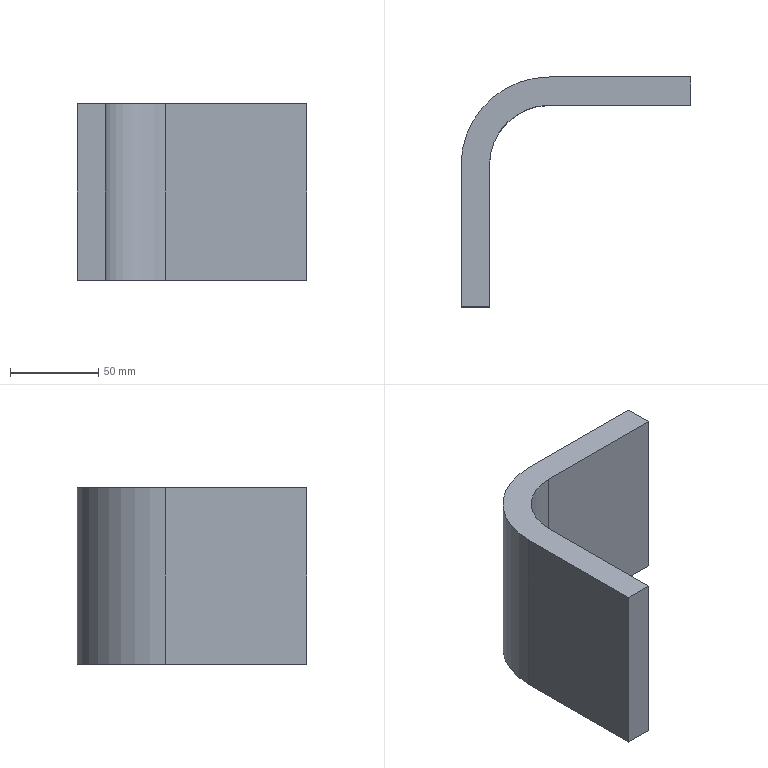Part | SolidWorks | features ExtruThin 1 | 1 solid | 10 faces | box 130 x 130 x 100 mm | volume 361558 mm3 | plane 8 | cylinder 2 | commonest cylinder face diameters 68 x1 100 x1
STEP:
#1=CARTESIAN_POINT('',(0.,-50.,0.));
#2=VERTEX_POINT('',#1);
#3=CARTESIAN_POINT('',(0.,-130.,0.));
#4=VERTEX_POINT('',#3);
#5=CARTESIAN_POINT('',(0.,-50.,0.));
#6=DIRECTION('',(0.,-1.,0.));
#7=VECTOR('',#6,1000.);
#8=LINE('',#5,#7);
#9=EDGE_CURVE('',#2,#4,#8,.T.);
#10=ORIENTED_EDGE('',*,*,#9,.T.);
#11=CARTESIAN_POINT('',(0.,-130.,100.));
#12=VERTEX_POINT('',#11);
#13=CARTESIAN_POINT('',(0.,-130.,100.));
#14=DIRECTION('',(0.,0.,-1.));
#15=VECTOR('',#14,1000.);
#16=LINE('',#13,#15);
#17=EDGE_CURVE('',#12,#4,#16,.T.);
#18=ORIENTED_EDGE('',*,*,#17,.F.);
#19=CARTESIAN_POINT('',(0.,-50.,100.));
#20=VERTEX_POINT('',#19);
#21=CARTESIAN_POINT('',(0.,-50.,100.));
#22=DIRECTION('',(0.,-1.,0.));
#23=VECTOR('',#22,1000.);
#24=LINE('',#21,#23);
#25=EDGE_CURVE('',#20,#12,#24,.T.);
#26=ORIENTED_EDGE('',*,*,#25,.F.);
#27=CARTESIAN_POINT('',(0.,-50.,100.));
#28=DIRECTION('',(0.,0.,-1.));
#29=VECTOR('',#28,1000.);
#30=LINE('',#27,#29);
#31=EDGE_CURVE('',#20,#2,#30,.T.);
#32=ORIENTED_EDGE('',*,*,#31,.T.);
#33=EDGE_LOOP('',(#10,#18,#26,#32));
#34=FACE_OUTER_BOUND('',#33,.T.);
#35=CARTESIAN_POINT('',(0.,-50.,100.));
#36=DIRECTION('',(1.,0.,0.));
#37=DIRECTION('',(0.,1.,0.));
#38=AXIS2_PLACEMENT_3D('',#35,#36,#37);
#39=PLANE('',#38);
#40=ADVANCED_FACE('',(#34),#39,.F.);
#41=CARTESIAN_POINT('',(16.,-130.,0.));
#42=VERTEX_POINT('',#41);
#43=CARTESIAN_POINT('',(16.,-130.,0.));
#44=DIRECTION('',(-1.,0.,0.));
#45=VECTOR('',#44,1000.);
#46=LINE('',#43,#45);
#47=EDGE_CURVE('',#42,#4,#46,.T.);
#48=ORIENTED_EDGE('',*,*,#47,.F.);
#49=CARTESIAN_POINT('',(16.,-130.,100.));
#50=VERTEX_POINT('',#49);
#51=CARTESIAN_POINT('',(16.,-130.,100.));
#52=DIRECTION('',(0.,0.,-1.));
#53=VECTOR('',#52,1000.);
#54=LINE('',#51,#53);
#55=EDGE_CURVE('',#50,#42,#54,.T.);
#56=ORIENTED_EDGE('',*,*,#55,.F.);
#57=CARTESIAN_POINT('',(16.,-130.,100.));
#58=DIRECTION('',(-1.,0.,0.));
#59=VECTOR('',#58,1000.);
#60=LINE('',#57,#59);
#61=EDGE_CURVE('',#50,#12,#60,.T.);
#62=ORIENTED_EDGE('',*,*,#61,.T.);
#63=ORIENTED_EDGE('',*,*,#17,.T.);
#64=EDGE_LOOP('',(#48,#56,#62,#63));
#65=FACE_OUTER_BOUND('',#64,.T.);
#66=CARTESIAN_POINT('',(16.,-130.,100.));
#67=DIRECTION('',(0.,-1.,0.));
#68=DIRECTION('',(0.,0.,-1.));
#69=AXIS2_PLACEMENT_3D('',#66,#67,#68);
#70=PLANE('',#69);
#71=ADVANCED_FACE('',(#65),#70,.T.);
#72=CARTESIAN_POINT('',(16.,-50.,0.));
#73=VERTEX_POINT('',#72);
#74=CARTESIAN_POINT('',(16.,-50.,0.));
#75=DIRECTION('',(0.,-1.,0.));
#76=VECTOR('',#75,1000.);
#77=LINE('',#74,#76);
#78=EDGE_CURVE('',#73,#42,#77,.T.);
#79=ORIENTED_EDGE('',*,*,#78,.F.);
#80=CARTESIAN_POINT('',(16.,-50.,100.));
#81=VERTEX_POINT('',#80);
#82=CARTESIAN_POINT('',(16.,-50.,100.));
#83=DIRECTION('',(0.,0.,-1.));
#84=VECTOR('',#83,1000.);
#85=LINE('',#82,#84);
#86=EDGE_CURVE('',#81,#73,#85,.T.);
#87=ORIENTED_EDGE('',*,*,#86,.F.);
#88=CARTESIAN_POINT('',(16.,-50.,100.));
#89=DIRECTION('',(0.,-1.,0.));
#90=VECTOR('',#89,1000.);
#91=LINE('',#88,#90);
#92=EDGE_CURVE('',#81,#50,#91,.T.);
#93=ORIENTED_EDGE('',*,*,#92,.T.);
#94=ORIENTED_EDGE('',*,*,#55,.T.);
#95=EDGE_LOOP('',(#79,#87,#93,#94));
#96=FACE_OUTER_BOUND('',#95,.T.);
#97=CARTESIAN_POINT('',(16.,-50.,100.));
#98=DIRECTION('',(1.,0.,0.));
#99=DIRECTION('',(0.,1.,0.));
#100=AXIS2_PLACEMENT_3D('',#97,#98,#99);
#101=PLANE('',#100);
#102=ADVANCED_FACE('',(#96),#101,.T.);
#103=CARTESIAN_POINT('',(50.,-16.,0.));
#104=VERTEX_POINT('',#103);
#105=CARTESIAN_POINT('',(50.,-50.,0.));
#106=DIRECTION('',(0.,0.,1.));
#107=DIRECTION('',(1.,0.,0.));
#108=AXIS2_PLACEMENT_3D('',#105,#106,#107);
#109=CIRCLE('',#108,34.);
#110=EDGE_CURVE('',#104,#73,#109,.T.);
#111=ORIENTED_EDGE('',*,*,#110,.F.);
#112=CARTESIAN_POINT('',(50.,-16.,100.));
#113=VERTEX_POINT('',#112);
#114=CARTESIAN_POINT('',(50.,-16.,100.));
#115=DIRECTION('',(0.,0.,-1.));
#116=VECTOR('',#115,1000.);
#117=LINE('',#114,#116);
#118=EDGE_CURVE('',#113,#104,#117,.T.);
#119=ORIENTED_EDGE('',*,*,#118,.F.);
#120=CARTESIAN_POINT('',(50.,-50.,100.));
#121=DIRECTION('',(0.,0.,1.));
#122=DIRECTION('',(1.,0.,0.));
#123=AXIS2_PLACEMENT_3D('',#120,#121,#122);
#124=CIRCLE('',#123,34.);
#125=EDGE_CURVE('',#113,#81,#124,.T.);
#126=ORIENTED_EDGE('',*,*,#125,.T.);
#127=ORIENTED_EDGE('',*,*,#86,.T.);
#128=EDGE_LOOP('',(#111,#119,#126,#127));
#129=FACE_OUTER_BOUND('',#128,.T.);
#130=CARTESIAN_POINT('',(50.,-50.,100.));
#131=DIRECTION('',(0.,0.,-1.));
#132=DIRECTION('',(-1.,0.,0.));
#133=AXIS2_PLACEMENT_3D('',#130,#131,#132);
#134=CYLINDRICAL_SURFACE('',#133,34.);
#135=ADVANCED_FACE('',(#129),#134,.F.);
#136=CARTESIAN_POINT('',(130.,-16.,0.));
#137=VERTEX_POINT('',#136);
#138=CARTESIAN_POINT('',(50.,-16.,0.));
#139=DIRECTION('',(-1.,0.,0.));
#140=VECTOR('',#139,1000.);
#141=LINE('',#138,#140);
#142=EDGE_CURVE('',#137,#104,#141,.T.);
#143=ORIENTED_EDGE('',*,*,#142,.F.);
#144=CARTESIAN_POINT('',(130.,-16.,100.));
#145=VERTEX_POINT('',#144);
#146=CARTESIAN_POINT('',(130.,-16.,100.));
#147=DIRECTION('',(0.,0.,-1.));
#148=VECTOR('',#147,1000.);
#149=LINE('',#146,#148);
#150=EDGE_CURVE('',#145,#137,#149,.T.);
#151=ORIENTED_EDGE('',*,*,#150,.F.);
#152=CARTESIAN_POINT('',(50.,-16.,100.));
#153=DIRECTION('',(-1.,0.,0.));
#154=VECTOR('',#153,1000.);
#155=LINE('',#152,#154);
#156=EDGE_CURVE('',#145,#113,#155,.T.);
#157=ORIENTED_EDGE('',*,*,#156,.T.);
#158=ORIENTED_EDGE('',*,*,#118,.T.);
#159=EDGE_LOOP('',(#143,#151,#157,#158));
#160=FACE_OUTER_BOUND('',#159,.T.);
#161=CARTESIAN_POINT('',(50.,-16.,100.));
#162=DIRECTION('',(0.,-1.,0.));
#163=DIRECTION('',(0.,0.,-1.));
#164=AXIS2_PLACEMENT_3D('',#161,#162,#163);
#165=PLANE('',#164);
#166=ADVANCED_FACE('',(#160),#165,.T.);
#167=CARTESIAN_POINT('',(130.,0.,0.));
#168=VERTEX_POINT('',#167);
#169=CARTESIAN_POINT('',(130.,0.,0.));
#170=DIRECTION('',(0.,-1.,0.));
#171=VECTOR('',#170,1000.);
#172=LINE('',#169,#171);
#173=EDGE_CURVE('',#168,#137,#172,.T.);
#174=ORIENTED_EDGE('',*,*,#173,.F.);
#175=CARTESIAN_POINT('',(130.,0.,100.));
#176=VERTEX_POINT('',#175);
#177=CARTESIAN_POINT('',(130.,0.,100.));
#178=DIRECTION('',(0.,0.,-1.));
#179=VECTOR('',#178,1000.);
#180=LINE('',#177,#179);
#181=EDGE_CURVE('',#176,#168,#180,.T.);
#182=ORIENTED_EDGE('',*,*,#181,.F.);
#183=CARTESIAN_POINT('',(130.,0.,100.));
#184=DIRECTION('',(0.,-1.,0.));
#185=VECTOR('',#184,1000.);
#186=LINE('',#183,#185);
#187=EDGE_CURVE('',#176,#145,#186,.T.);
#188=ORIENTED_EDGE('',*,*,#187,.T.);
#189=ORIENTED_EDGE('',*,*,#150,.T.);
#190=EDGE_LOOP('',(#174,#182,#188,#189));
#191=FACE_OUTER_BOUND('',#190,.T.);
#192=CARTESIAN_POINT('',(130.,0.,100.));
#193=DIRECTION('',(1.,0.,0.));
#194=DIRECTION('',(0.,0.,-1.));
#195=AXIS2_PLACEMENT_3D('',#192,#193,#194);
#196=PLANE('',#195);
#197=ADVANCED_FACE('',(#191),#196,.T.);
#198=CARTESIAN_POINT('',(50.,0.,0.));
#199=VERTEX_POINT('',#198);
#200=CARTESIAN_POINT('',(50.,0.,0.));
#201=DIRECTION('',(-1.,0.,0.));
#202=VECTOR('',#201,1000.);
#203=LINE('',#200,#202);
#204=EDGE_CURVE('',#168,#199,#203,.T.);
#205=ORIENTED_EDGE('',*,*,#204,.T.);
#206=CARTESIAN_POINT('',(50.,0.,100.));
#207=VERTEX_POINT('',#206);
#208=CARTESIAN_POINT('',(50.,0.,100.));
#209=DIRECTION('',(0.,0.,-1.));
#210=VECTOR('',#209,1000.);
#211=LINE('',#208,#210);
#212=EDGE_CURVE('',#207,#199,#211,.T.);
#213=ORIENTED_EDGE('',*,*,#212,.F.);
#214=CARTESIAN_POINT('',(50.,0.,100.));
#215=DIRECTION('',(-1.,0.,0.));
#216=VECTOR('',#215,1000.);
#217=LINE('',#214,#216);
#218=EDGE_CURVE('',#176,#207,#217,.T.);
#219=ORIENTED_EDGE('',*,*,#218,.F.);
#220=ORIENTED_EDGE('',*,*,#181,.T.);
#221=EDGE_LOOP('',(#205,#213,#219,#220));
#222=FACE_OUTER_BOUND('',#221,.T.);
#223=CARTESIAN_POINT('',(50.,0.,100.));
#224=DIRECTION('',(0.,-1.,0.));
#225=DIRECTION('',(0.,0.,-1.));
#226=AXIS2_PLACEMENT_3D('',#223,#224,#225);
#227=PLANE('',#226);
#228=ADVANCED_FACE('',(#222),#227,.F.);
#229=CARTESIAN_POINT('',(50.,-50.,0.));
#230=DIRECTION('',(0.,0.,1.));
#231=DIRECTION('',(1.,0.,0.));
#232=AXIS2_PLACEMENT_3D('',#229,#230,#231);
#233=CIRCLE('',#232,50.);
#234=EDGE_CURVE('',#199,#2,#233,.T.);
#235=ORIENTED_EDGE('',*,*,#234,.T.);
#236=ORIENTED_EDGE('',*,*,#31,.F.);
#237=CARTESIAN_POINT('',(50.,-50.,100.));
#238=DIRECTION('',(0.,0.,1.));
#239=DIRECTION('',(1.,0.,0.));
#240=AXIS2_PLACEMENT_3D('',#237,#238,#239);
#241=CIRCLE('',#240,50.);
#242=EDGE_CURVE('',#207,#20,#241,.T.);
#243=ORIENTED_EDGE('',*,*,#242,.F.);
#244=ORIENTED_EDGE('',*,*,#212,.T.);
#245=EDGE_LOOP('',(#235,#236,#243,#244));
#246=FACE_OUTER_BOUND('',#245,.T.);
#247=CARTESIAN_POINT('',(50.,-50.,100.));
#248=DIRECTION('',(0.,0.,-1.));
#249=DIRECTION('',(-1.,0.,0.));
#250=AXIS2_PLACEMENT_3D('',#247,#248,#249);
#251=CYLINDRICAL_SURFACE('',#250,50.);
#252=ADVANCED_FACE('',(#246),#251,.T.);
#253=ORIENTED_EDGE('',*,*,#25,.T.);
#254=ORIENTED_EDGE('',*,*,#61,.F.);
#255=ORIENTED_EDGE('',*,*,#92,.F.);
#256=ORIENTED_EDGE('',*,*,#125,.F.);
#257=ORIENTED_EDGE('',*,*,#156,.F.);
#258=ORIENTED_EDGE('',*,*,#187,.F.);
#259=ORIENTED_EDGE('',*,*,#218,.T.);
#260=ORIENTED_EDGE('',*,*,#242,.T.);
#261=EDGE_LOOP('',(#253,#254,#255,#256,#257,#258,#259,#260));
#262=FACE_OUTER_BOUND('',#261,.T.);
#263=CARTESIAN_POINT('',(50.,-50.,100.));
#264=DIRECTION('',(0.,0.,1.));
#265=DIRECTION('',(1.,0.,0.));
#266=AXIS2_PLACEMENT_3D('',#263,#264,#265);
#267=PLANE('',#266);
#268=ADVANCED_FACE('',(#262),#267,.T.);
#269=ORIENTED_EDGE('',*,*,#9,.F.);
#270=ORIENTED_EDGE('',*,*,#234,.F.);
#271=ORIENTED_EDGE('',*,*,#204,.F.);
#272=ORIENTED_EDGE('',*,*,#173,.T.);
#273=ORIENTED_EDGE('',*,*,#142,.T.);
#274=ORIENTED_EDGE('',*,*,#110,.T.);
#275=ORIENTED_EDGE('',*,*,#78,.T.);
#276=ORIENTED_EDGE('',*,*,#47,.T.);
#277=EDGE_LOOP('',(#269,#270,#271,#272,#273,#274,#275,#276));
#278=FACE_OUTER_BOUND('',#277,.T.);
#279=CARTESIAN_POINT('',(50.,-50.,0.));
#280=DIRECTION('',(0.,0.,1.));
#281=DIRECTION('',(1.,0.,0.));
#282=AXIS2_PLACEMENT_3D('',#279,#280,#281);
#283=PLANE('',#282);
#284=ADVANCED_FACE('',(#278),#283,.F.);
#285=CLOSED_SHELL('',(#40,#71,#102,#135,#166,#197,#228,#252,#268,#284));
#286=MANIFOLD_SOLID_BREP('',#285);
#287=CARTESIAN_POINT('',(0.,0.,0.));
#288=DIRECTION('',(0.,0.,1.));
#289=DIRECTION('',(1.,0.,0.));
#290=AXIS2_PLACEMENT_3D('',#287,#288,#289);
#291=(LENGTH_UNIT()NAMED_UNIT(*)SI_UNIT(.MILLI.,.METRE.));
#292=UNCERTAINTY_MEASURE_WITH_UNIT(LENGTH_MEASURE(0.00001),#291,'','');
#293=(NAMED_UNIT(*)PLANE_ANGLE_UNIT()SI_UNIT($,.RADIAN.));
#294=(NAMED_UNIT(*)SI_UNIT($,.STERADIAN.)SOLID_ANGLE_UNIT());
#295=(GEOMETRIC_REPRESENTATION_CONTEXT(3)GLOBAL_UNCERTAINTY_ASSIGNED_CONTEXT((#292))GLOBAL_UNIT_ASSIGNED_CONTEXT((#291,#293,#294))REPRESENTATION_CONTEXT('',''));
#296=ADVANCED_BREP_SHAPE_REPRESENTATION('',(#286,#290),#295);